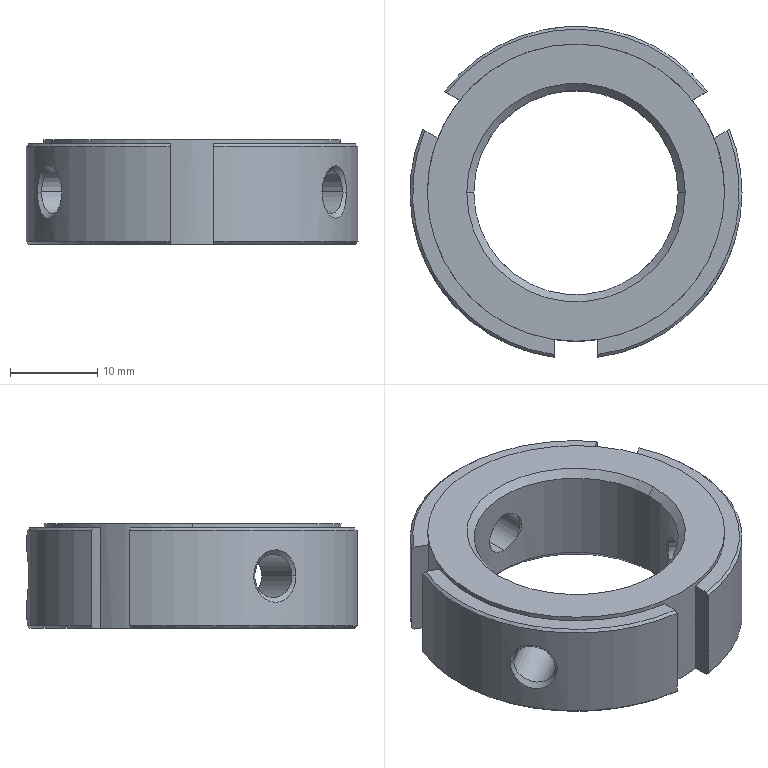Part | SolidWorks | features BaseBody 1 | 1 solid | 50 faces | box 38 x 37.835 x 12 mm | volume 7518 mm3 | cone 25 | cylinder 14 | plane 11 | commonest cylinder face diameters 4.917 x6 38 x4 23.376 x2 34 x2